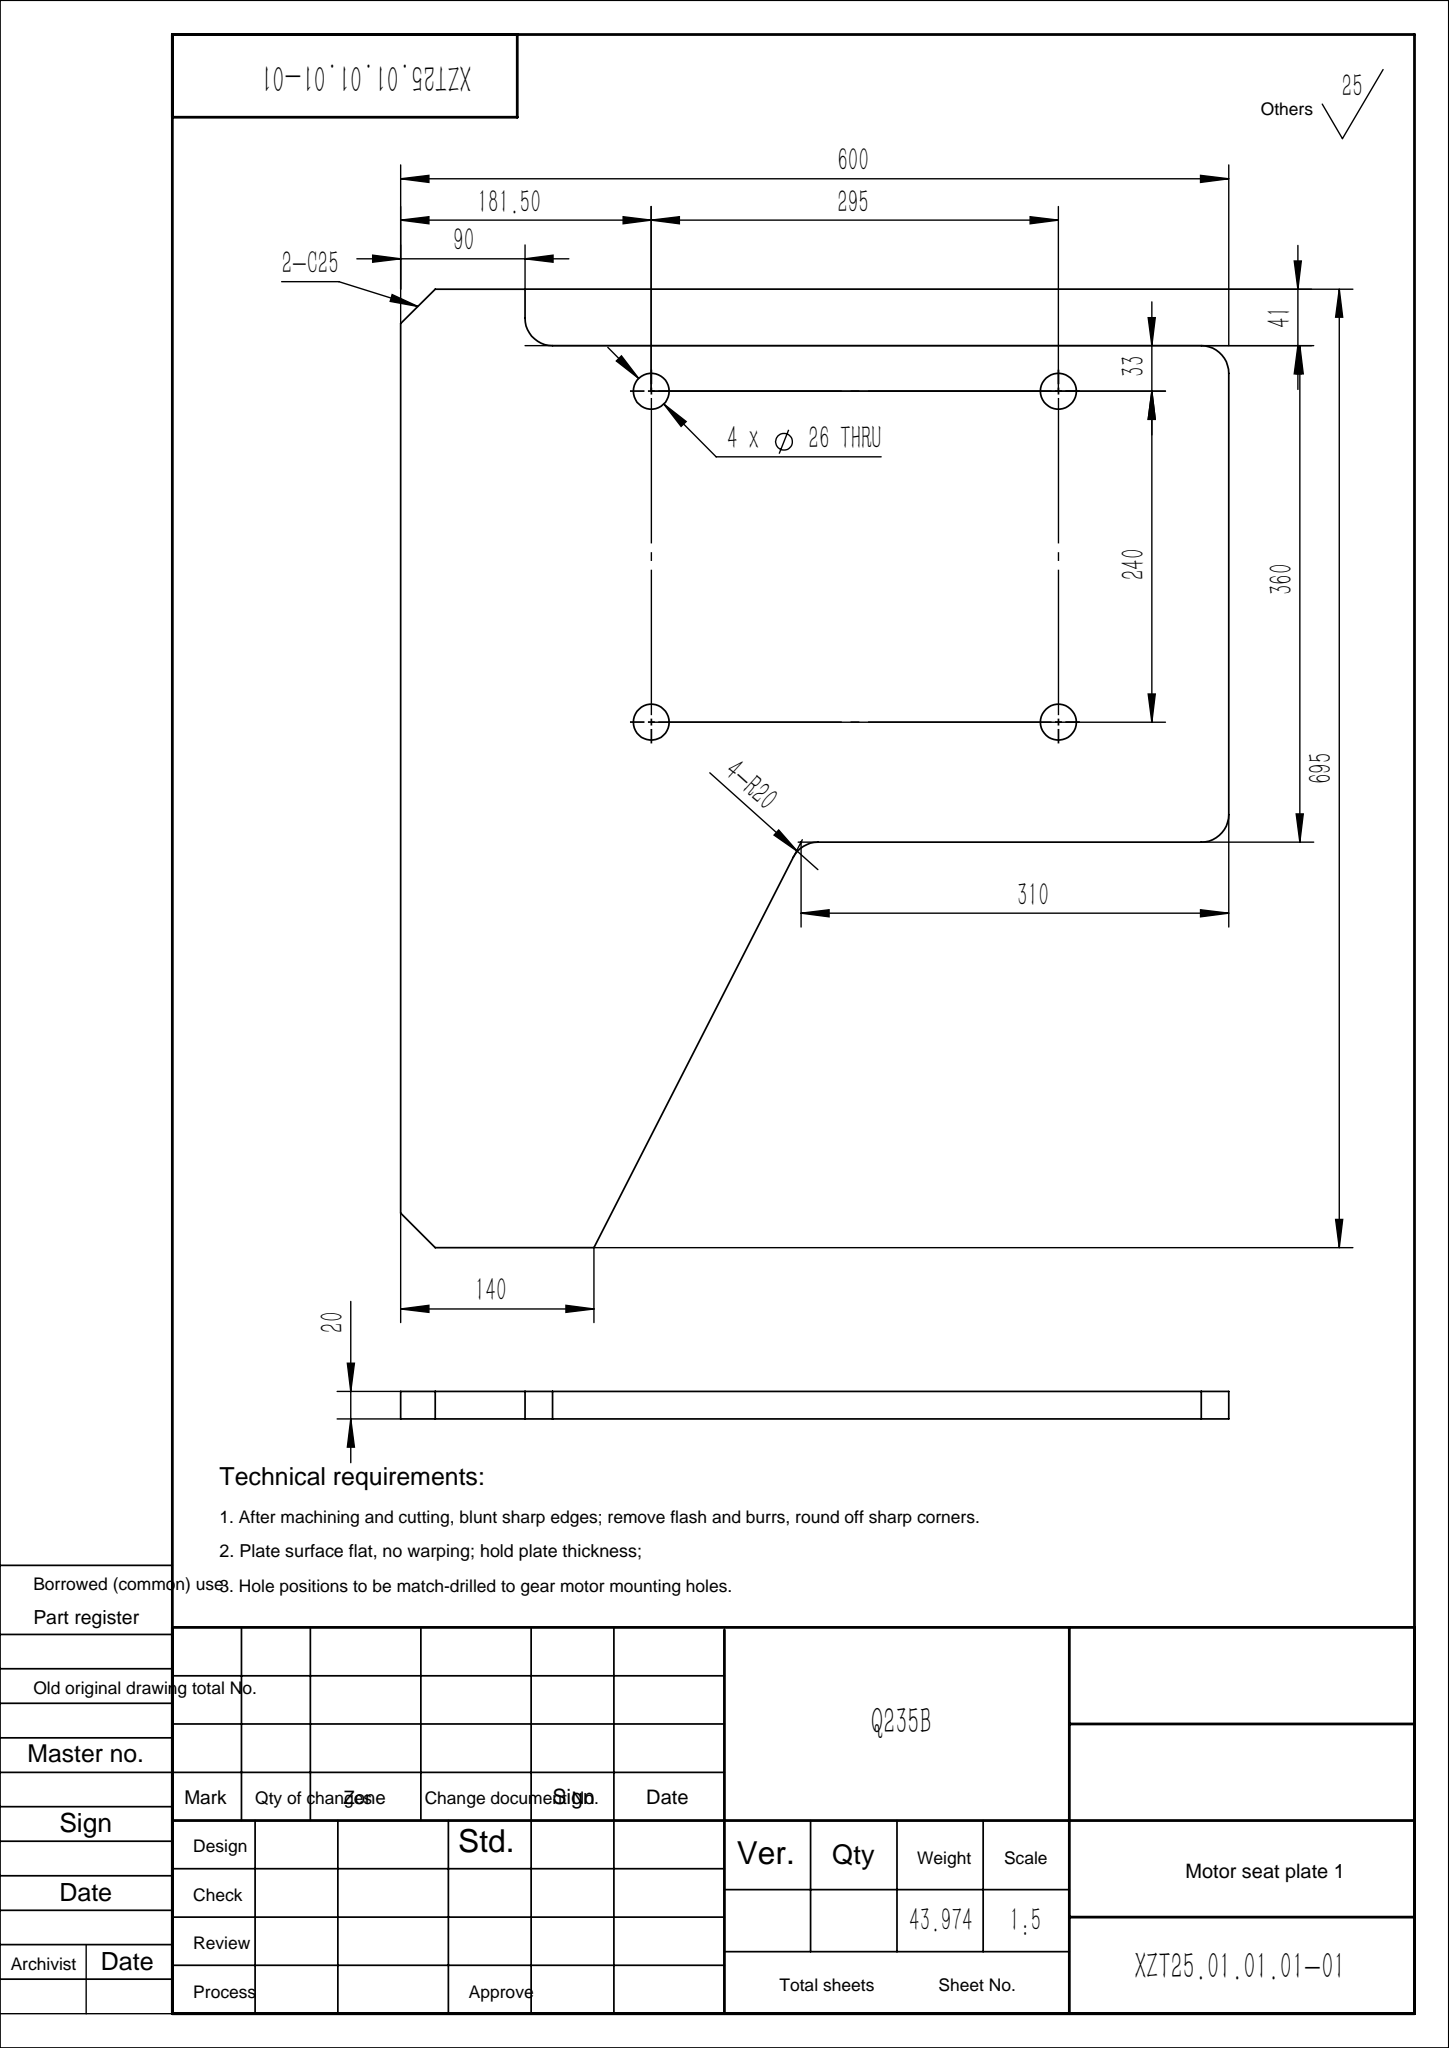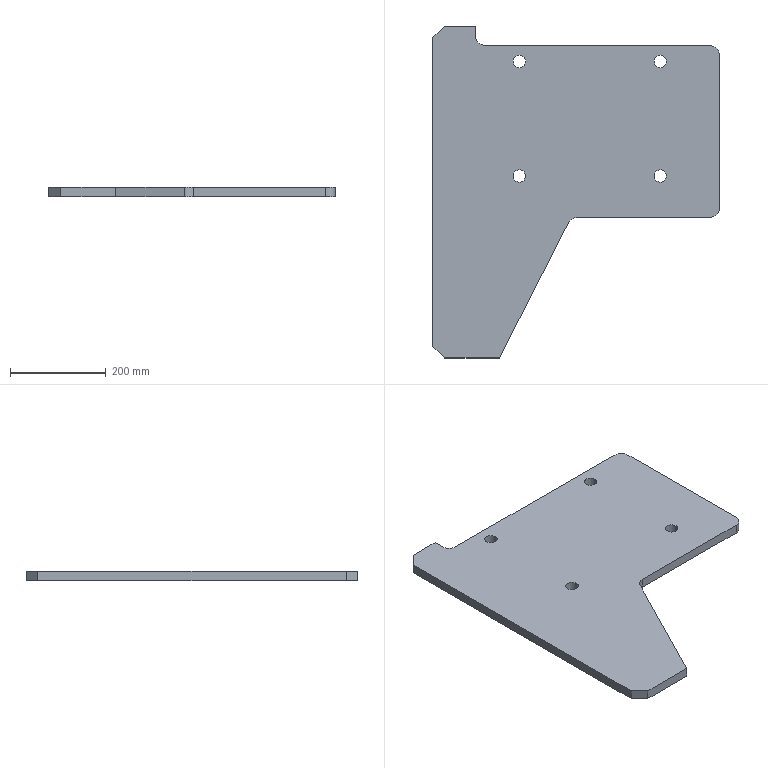Part | SolidWorks | features Chamfer 1, Extrusion 1, Fillet 1, HoleWzd 1 | 1 solid | 24 faces | box 600 x 695 x 20 mm | volume 5601812 mm3 | cylinder 12 | plane 12 | commonest cylinder face diameters 26 x8 40 x4
STEP:
#1=CARTESIAN_POINT('',(194.5,621.,-10.));
#2=VERTEX_POINT('',#1);
#3=CARTESIAN_POINT('',(168.5,621.,-10.));
#4=VERTEX_POINT('',#3);
#5=CARTESIAN_POINT('',(181.5,621.,-10.));
#6=DIRECTION('',(0.,0.,-1.));
#7=DIRECTION('',(-1.,0.,0.));
#8=AXIS2_PLACEMENT_3D('',#5,#6,#7);
#9=CIRCLE('',#8,13.);
#10=EDGE_CURVE('',#2,#4,#9,.T.);
#11=ORIENTED_EDGE('',*,*,#10,.T.);
#12=CARTESIAN_POINT('',(168.5,621.,10.));
#13=VERTEX_POINT('',#12);
#14=CARTESIAN_POINT('',(168.5,621.,10.));
#15=DIRECTION('',(0.,0.,1.));
#16=VECTOR('',#15,1000.);
#17=LINE('',#14,#16);
#18=EDGE_CURVE('',#4,#13,#17,.T.);
#19=ORIENTED_EDGE('',*,*,#18,.T.);
#20=CARTESIAN_POINT('',(194.5,621.,10.));
#21=VERTEX_POINT('',#20);
#22=CARTESIAN_POINT('',(181.5,621.,10.));
#23=DIRECTION('',(0.,0.,1.));
#24=DIRECTION('',(1.,0.,0.));
#25=AXIS2_PLACEMENT_3D('',#22,#23,#24);
#26=CIRCLE('',#25,13.);
#27=EDGE_CURVE('',#13,#21,#26,.T.);
#28=ORIENTED_EDGE('',*,*,#27,.T.);
#29=CARTESIAN_POINT('',(194.5,621.,10.));
#30=DIRECTION('',(0.,0.,1.));
#31=VECTOR('',#30,1000.);
#32=LINE('',#29,#31);
#33=EDGE_CURVE('',#2,#21,#32,.T.);
#34=ORIENTED_EDGE('',*,*,#33,.F.);
#35=EDGE_LOOP('',(#11,#19,#28,#34));
#36=FACE_OUTER_BOUND('',#35,.T.);
#37=CARTESIAN_POINT('',(181.5,621.,10.));
#38=DIRECTION('',(0.,0.,1.));
#39=DIRECTION('',(1.,0.,0.));
#40=AXIS2_PLACEMENT_3D('',#37,#38,#39);
#41=CYLINDRICAL_SURFACE('',#40,13.);
#42=ADVANCED_FACE('',(#36),#41,.F.);
#43=CARTESIAN_POINT('',(489.5,621.,-10.));
#44=VERTEX_POINT('',#43);
#45=CARTESIAN_POINT('',(463.5,621.,-10.));
#46=VERTEX_POINT('',#45);
#47=CARTESIAN_POINT('',(476.5,621.,-10.));
#48=DIRECTION('',(0.,0.,-1.));
#49=DIRECTION('',(-1.,0.,0.));
#50=AXIS2_PLACEMENT_3D('',#47,#48,#49);
#51=CIRCLE('',#50,13.);
#52=EDGE_CURVE('',#44,#46,#51,.T.);
#53=ORIENTED_EDGE('',*,*,#52,.T.);
#54=CARTESIAN_POINT('',(463.5,621.,10.));
#55=VERTEX_POINT('',#54);
#56=CARTESIAN_POINT('',(463.5,621.,10.));
#57=DIRECTION('',(0.,0.,1.));
#58=VECTOR('',#57,1000.);
#59=LINE('',#56,#58);
#60=EDGE_CURVE('',#46,#55,#59,.T.);
#61=ORIENTED_EDGE('',*,*,#60,.T.);
#62=CARTESIAN_POINT('',(489.5,621.,10.));
#63=VERTEX_POINT('',#62);
#64=CARTESIAN_POINT('',(476.5,621.,10.));
#65=DIRECTION('',(0.,0.,1.));
#66=DIRECTION('',(1.,0.,0.));
#67=AXIS2_PLACEMENT_3D('',#64,#65,#66);
#68=CIRCLE('',#67,13.);
#69=EDGE_CURVE('',#55,#63,#68,.T.);
#70=ORIENTED_EDGE('',*,*,#69,.T.);
#71=CARTESIAN_POINT('',(489.5,621.,10.));
#72=DIRECTION('',(0.,0.,1.));
#73=VECTOR('',#72,1000.);
#74=LINE('',#71,#73);
#75=EDGE_CURVE('',#44,#63,#74,.T.);
#76=ORIENTED_EDGE('',*,*,#75,.F.);
#77=EDGE_LOOP('',(#53,#61,#70,#76));
#78=FACE_OUTER_BOUND('',#77,.T.);
#79=CARTESIAN_POINT('',(476.5,621.,10.));
#80=DIRECTION('',(0.,0.,1.));
#81=DIRECTION('',(1.,0.,0.));
#82=AXIS2_PLACEMENT_3D('',#79,#80,#81);
#83=CYLINDRICAL_SURFACE('',#82,13.);
#84=ADVANCED_FACE('',(#78),#83,.F.);
#85=CARTESIAN_POINT('',(489.5,381.,-10.));
#86=VERTEX_POINT('',#85);
#87=CARTESIAN_POINT('',(463.5,381.,-10.));
#88=VERTEX_POINT('',#87);
#89=CARTESIAN_POINT('',(476.5,381.,-10.));
#90=DIRECTION('',(0.,0.,-1.));
#91=DIRECTION('',(-1.,0.,0.));
#92=AXIS2_PLACEMENT_3D('',#89,#90,#91);
#93=CIRCLE('',#92,13.);
#94=EDGE_CURVE('',#86,#88,#93,.T.);
#95=ORIENTED_EDGE('',*,*,#94,.T.);
#96=CARTESIAN_POINT('',(463.5,381.,10.));
#97=VERTEX_POINT('',#96);
#98=CARTESIAN_POINT('',(463.5,381.,10.));
#99=DIRECTION('',(0.,0.,1.));
#100=VECTOR('',#99,1000.);
#101=LINE('',#98,#100);
#102=EDGE_CURVE('',#88,#97,#101,.T.);
#103=ORIENTED_EDGE('',*,*,#102,.T.);
#104=CARTESIAN_POINT('',(489.5,381.,10.));
#105=VERTEX_POINT('',#104);
#106=CARTESIAN_POINT('',(476.5,381.,10.));
#107=DIRECTION('',(0.,0.,1.));
#108=DIRECTION('',(1.,0.,0.));
#109=AXIS2_PLACEMENT_3D('',#106,#107,#108);
#110=CIRCLE('',#109,13.);
#111=EDGE_CURVE('',#97,#105,#110,.T.);
#112=ORIENTED_EDGE('',*,*,#111,.T.);
#113=CARTESIAN_POINT('',(489.5,381.,10.));
#114=DIRECTION('',(0.,0.,1.));
#115=VECTOR('',#114,1000.);
#116=LINE('',#113,#115);
#117=EDGE_CURVE('',#86,#105,#116,.T.);
#118=ORIENTED_EDGE('',*,*,#117,.F.);
#119=EDGE_LOOP('',(#95,#103,#112,#118));
#120=FACE_OUTER_BOUND('',#119,.T.);
#121=CARTESIAN_POINT('',(476.5,381.,10.));
#122=DIRECTION('',(0.,0.,1.));
#123=DIRECTION('',(1.,0.,0.));
#124=AXIS2_PLACEMENT_3D('',#121,#122,#123);
#125=CYLINDRICAL_SURFACE('',#124,13.);
#126=ADVANCED_FACE('',(#120),#125,.F.);
#127=CARTESIAN_POINT('',(194.5,381.,-10.));
#128=VERTEX_POINT('',#127);
#129=CARTESIAN_POINT('',(168.5,381.,-10.));
#130=VERTEX_POINT('',#129);
#131=CARTESIAN_POINT('',(181.5,381.,-10.));
#132=DIRECTION('',(0.,0.,-1.));
#133=DIRECTION('',(-1.,0.,0.));
#134=AXIS2_PLACEMENT_3D('',#131,#132,#133);
#135=CIRCLE('',#134,13.);
#136=EDGE_CURVE('',#128,#130,#135,.T.);
#137=ORIENTED_EDGE('',*,*,#136,.T.);
#138=CARTESIAN_POINT('',(168.5,381.,10.));
#139=VERTEX_POINT('',#138);
#140=CARTESIAN_POINT('',(168.5,381.,10.));
#141=DIRECTION('',(0.,0.,1.));
#142=VECTOR('',#141,1000.);
#143=LINE('',#140,#142);
#144=EDGE_CURVE('',#130,#139,#143,.T.);
#145=ORIENTED_EDGE('',*,*,#144,.T.);
#146=CARTESIAN_POINT('',(194.5,381.,10.));
#147=VERTEX_POINT('',#146);
#148=CARTESIAN_POINT('',(181.5,381.,10.));
#149=DIRECTION('',(0.,0.,1.));
#150=DIRECTION('',(1.,0.,0.));
#151=AXIS2_PLACEMENT_3D('',#148,#149,#150);
#152=CIRCLE('',#151,13.);
#153=EDGE_CURVE('',#139,#147,#152,.T.);
#154=ORIENTED_EDGE('',*,*,#153,.T.);
#155=CARTESIAN_POINT('',(194.5,381.,10.));
#156=DIRECTION('',(0.,0.,1.));
#157=VECTOR('',#156,1000.);
#158=LINE('',#155,#157);
#159=EDGE_CURVE('',#128,#147,#158,.T.);
#160=ORIENTED_EDGE('',*,*,#159,.F.);
#161=EDGE_LOOP('',(#137,#145,#154,#160));
#162=FACE_OUTER_BOUND('',#161,.T.);
#163=CARTESIAN_POINT('',(181.5,381.,10.));
#164=DIRECTION('',(0.,0.,1.));
#165=DIRECTION('',(1.,0.,0.));
#166=AXIS2_PLACEMENT_3D('',#163,#164,#165);
#167=CYLINDRICAL_SURFACE('',#166,13.);
#168=ADVANCED_FACE('',(#162),#167,.F.);
#169=CARTESIAN_POINT('',(476.5,381.,10.));
#170=DIRECTION('',(0.,0.,1.));
#171=DIRECTION('',(1.,0.,0.));
#172=AXIS2_PLACEMENT_3D('',#169,#170,#171);
#173=CIRCLE('',#172,13.);
#174=EDGE_CURVE('',#105,#97,#173,.T.);
#175=ORIENTED_EDGE('',*,*,#174,.F.);
#176=ORIENTED_EDGE('',*,*,#111,.F.);
#177=EDGE_LOOP('',(#175,#176));
#178=FACE_BOUND('',#177,.T.);
#179=CARTESIAN_POINT('',(181.5,381.,10.));
#180=DIRECTION('',(0.,0.,1.));
#181=DIRECTION('',(1.,0.,0.));
#182=AXIS2_PLACEMENT_3D('',#179,#180,#181);
#183=CIRCLE('',#182,13.);
#184=EDGE_CURVE('',#147,#139,#183,.T.);
#185=ORIENTED_EDGE('',*,*,#184,.F.);
#186=ORIENTED_EDGE('',*,*,#153,.F.);
#187=EDGE_LOOP('',(#185,#186));
#188=FACE_BOUND('',#187,.T.);
#189=CARTESIAN_POINT('',(302.249,294.,10.));
#190=VERTEX_POINT('',#189);
#191=CARTESIAN_POINT('',(580.,294.,10.));
#192=VERTEX_POINT('',#191);
#193=CARTESIAN_POINT('',(600.,294.,10.));
#194=DIRECTION('',(1.,0.,0.));
#195=VECTOR('',#194,1000.);
#196=LINE('',#193,#195);
#197=EDGE_CURVE('',#190,#192,#196,.T.);
#198=ORIENTED_EDGE('',*,*,#197,.T.);
#199=CARTESIAN_POINT('',(600.,314.,10.));
#200=VERTEX_POINT('',#199);
#201=CARTESIAN_POINT('',(580.,314.,10.));
#202=DIRECTION('',(0.,0.,1.));
#203=DIRECTION('',(-1.,0.,0.));
#204=AXIS2_PLACEMENT_3D('',#201,#202,#203);
#205=CIRCLE('',#204,20.);
#206=EDGE_CURVE('',#192,#200,#205,.T.);
#207=ORIENTED_EDGE('',*,*,#206,.T.);
#208=CARTESIAN_POINT('',(600.,634.,10.));
#209=VERTEX_POINT('',#208);
#210=CARTESIAN_POINT('',(600.,654.,10.));
#211=DIRECTION('',(0.,1.,0.));
#212=VECTOR('',#211,1000.);
#213=LINE('',#210,#212);
#214=EDGE_CURVE('',#200,#209,#213,.T.);
#215=ORIENTED_EDGE('',*,*,#214,.T.);
#216=CARTESIAN_POINT('',(580.,654.,10.));
#217=VERTEX_POINT('',#216);
#218=CARTESIAN_POINT('',(580.,634.,10.));
#219=DIRECTION('',(0.,0.,1.));
#220=DIRECTION('',(-1.,0.,0.));
#221=AXIS2_PLACEMENT_3D('',#218,#219,#220);
#222=CIRCLE('',#221,20.);
#223=EDGE_CURVE('',#209,#217,#222,.T.);
#224=ORIENTED_EDGE('',*,*,#223,.T.);
#225=CARTESIAN_POINT('',(110.,654.,10.));
#226=VERTEX_POINT('',#225);
#227=CARTESIAN_POINT('',(90.,654.,10.));
#228=DIRECTION('',(-1.,0.,0.));
#229=VECTOR('',#228,1000.);
#230=LINE('',#227,#229);
#231=EDGE_CURVE('',#217,#226,#230,.T.);
#232=ORIENTED_EDGE('',*,*,#231,.T.);
#233=CARTESIAN_POINT('',(90.,674.,10.));
#234=VERTEX_POINT('',#233);
#235=CARTESIAN_POINT('',(110.,674.,10.));
#236=DIRECTION('',(0.,0.,-1.));
#237=DIRECTION('',(-1.,0.,0.));
#238=AXIS2_PLACEMENT_3D('',#235,#236,#237);
#239=CIRCLE('',#238,20.);
#240=EDGE_CURVE('',#226,#234,#239,.T.);
#241=ORIENTED_EDGE('',*,*,#240,.T.);
#242=CARTESIAN_POINT('',(90.,695.,10.));
#243=VERTEX_POINT('',#242);
#244=CARTESIAN_POINT('',(90.,695.,10.));
#245=DIRECTION('',(0.,1.,0.));
#246=VECTOR('',#245,1000.);
#247=LINE('',#244,#246);
#248=EDGE_CURVE('',#234,#243,#247,.T.);
#249=ORIENTED_EDGE('',*,*,#248,.T.);
#250=CARTESIAN_POINT('',(25.,695.,10.));
#251=VERTEX_POINT('',#250);
#252=CARTESIAN_POINT('',(0.,695.,10.));
#253=DIRECTION('',(-1.,0.,0.));
#254=VECTOR('',#253,1000.);
#255=LINE('',#252,#254);
#256=EDGE_CURVE('',#243,#251,#255,.T.);
#257=ORIENTED_EDGE('',*,*,#256,.T.);
#258=CARTESIAN_POINT('',(0.,670.,10.));
#259=VERTEX_POINT('',#258);
#260=CARTESIAN_POINT('',(0.,670.,10.));
#261=DIRECTION('',(-0.7071,-0.7071,0.));
#262=VECTOR('',#261,1000.);
#263=LINE('',#260,#262);
#264=EDGE_CURVE('',#251,#259,#263,.T.);
#265=ORIENTED_EDGE('',*,*,#264,.T.);
#266=CARTESIAN_POINT('',(0.,25.,10.));
#267=VERTEX_POINT('',#266);
#268=CARTESIAN_POINT('',(0.,0.,10.));
#269=DIRECTION('',(0.,-1.,0.));
#270=VECTOR('',#269,1000.);
#271=LINE('',#268,#270);
#272=EDGE_CURVE('',#259,#267,#271,.T.);
#273=ORIENTED_EDGE('',*,*,#272,.T.);
#274=CARTESIAN_POINT('',(25.,0.,10.));
#275=VERTEX_POINT('',#274);
#276=CARTESIAN_POINT('',(25.,0.,10.));
#277=DIRECTION('',(0.7071,-0.7071,0.));
#278=VECTOR('',#277,1000.);
#279=LINE('',#276,#278);
#280=EDGE_CURVE('',#267,#275,#279,.T.);
#281=ORIENTED_EDGE('',*,*,#280,.T.);
#282=CARTESIAN_POINT('',(140.,0.,10.));
#283=VERTEX_POINT('',#282);
#284=CARTESIAN_POINT('',(140.,0.,10.));
#285=DIRECTION('',(1.,0.,0.));
#286=VECTOR('',#285,1000.);
#287=LINE('',#284,#286);
#288=EDGE_CURVE('',#275,#283,#287,.T.);
#289=ORIENTED_EDGE('',*,*,#288,.T.);
#290=CARTESIAN_POINT('',(284.433,283.089,10.));
#291=VERTEX_POINT('',#290);
#292=CARTESIAN_POINT('',(290.,294.,10.));
#293=DIRECTION('',(0.4545,0.8908,0.));
#294=VECTOR('',#293,1000.);
#295=LINE('',#292,#294);
#296=EDGE_CURVE('',#283,#291,#295,.T.);
#297=ORIENTED_EDGE('',*,*,#296,.T.);
#298=CARTESIAN_POINT('',(302.249,274.,10.));
#299=DIRECTION('',(0.,0.,-1.));
#300=DIRECTION('',(-1.,0.,0.));
#301=AXIS2_PLACEMENT_3D('',#298,#299,#300);
#302=CIRCLE('',#301,20.);
#303=EDGE_CURVE('',#291,#190,#302,.T.);
#304=ORIENTED_EDGE('',*,*,#303,.T.);
#305=EDGE_LOOP('',(#198,#207,#215,#224,#232,#241,#249,#257,#265,#273,#281,#289,#297,#304));
#306=FACE_OUTER_BOUND('',#305,.T.);
#307=CARTESIAN_POINT('',(476.5,621.,10.));
#308=DIRECTION('',(0.,0.,1.));
#309=DIRECTION('',(1.,0.,0.));
#310=AXIS2_PLACEMENT_3D('',#307,#308,#309);
#311=CIRCLE('',#310,13.);
#312=EDGE_CURVE('',#63,#55,#311,.T.);
#313=ORIENTED_EDGE('',*,*,#312,.F.);
#314=ORIENTED_EDGE('',*,*,#69,.F.);
#315=EDGE_LOOP('',(#313,#314));
#316=FACE_BOUND('',#315,.T.);
#317=CARTESIAN_POINT('',(181.5,621.,10.));
#318=DIRECTION('',(0.,0.,1.));
#319=DIRECTION('',(1.,0.,0.));
#320=AXIS2_PLACEMENT_3D('',#317,#318,#319);
#321=CIRCLE('',#320,13.);
#322=EDGE_CURVE('',#21,#13,#321,.T.);
#323=ORIENTED_EDGE('',*,*,#322,.F.);
#324=ORIENTED_EDGE('',*,*,#27,.F.);
#325=EDGE_LOOP('',(#323,#324));
#326=FACE_BOUND('',#325,.T.);
#327=CARTESIAN_POINT('',(0.,0.,10.));
#328=DIRECTION('',(0.,0.,-1.));
#329=DIRECTION('',(-1.,0.,0.));
#330=AXIS2_PLACEMENT_3D('',#327,#328,#329);
#331=PLANE('',#330);
#332=ADVANCED_FACE('',(#178,#188,#306,#316,#326),#331,.F.);
#333=ORIENTED_EDGE('',*,*,#288,.F.);
#334=CARTESIAN_POINT('',(25.,0.,-10.));
#335=VERTEX_POINT('',#334);
#336=CARTESIAN_POINT('',(25.,0.,10.));
#337=DIRECTION('',(0.,0.,-1.));
#338=VECTOR('',#337,1000.);
#339=LINE('',#336,#338);
#340=EDGE_CURVE('',#275,#335,#339,.T.);
#341=ORIENTED_EDGE('',*,*,#340,.T.);
#342=CARTESIAN_POINT('',(140.,0.,-10.));
#343=VERTEX_POINT('',#342);
#344=CARTESIAN_POINT('',(140.,0.,-10.));
#345=DIRECTION('',(1.,0.,0.));
#346=VECTOR('',#345,1000.);
#347=LINE('',#344,#346);
#348=EDGE_CURVE('',#335,#343,#347,.T.);
#349=ORIENTED_EDGE('',*,*,#348,.T.);
#350=CARTESIAN_POINT('',(140.,0.,10.));
#351=DIRECTION('',(0.,0.,-1.));
#352=VECTOR('',#351,1000.);
#353=LINE('',#350,#352);
#354=EDGE_CURVE('',#283,#343,#353,.T.);
#355=ORIENTED_EDGE('',*,*,#354,.F.);
#356=EDGE_LOOP('',(#333,#341,#349,#355));
#357=FACE_OUTER_BOUND('',#356,.T.);
#358=CARTESIAN_POINT('',(140.,0.,10.));
#359=DIRECTION('',(0.,1.,0.));
#360=DIRECTION('',(0.,0.,1.));
#361=AXIS2_PLACEMENT_3D('',#358,#359,#360);
#362=PLANE('',#361);
#363=ADVANCED_FACE('',(#357),#362,.F.);
#364=CARTESIAN_POINT('',(284.433,283.089,-10.));
#365=VERTEX_POINT('',#364);
#366=CARTESIAN_POINT('',(290.,294.,-10.));
#367=DIRECTION('',(0.4545,0.8908,0.));
#368=VECTOR('',#367,1000.);
#369=LINE('',#366,#368);
#370=EDGE_CURVE('',#343,#365,#369,.T.);
#371=ORIENTED_EDGE('',*,*,#370,.T.);
#372=CARTESIAN_POINT('',(284.433,283.089,10.));
#373=DIRECTION('',(0.,0.,1.));
#374=VECTOR('',#373,1000.);
#375=LINE('',#372,#374);
#376=EDGE_CURVE('',#365,#291,#375,.T.);
#377=ORIENTED_EDGE('',*,*,#376,.T.);
#378=ORIENTED_EDGE('',*,*,#296,.F.);
#379=ORIENTED_EDGE('',*,*,#354,.T.);
#380=EDGE_LOOP('',(#371,#377,#378,#379));
#381=FACE_OUTER_BOUND('',#380,.T.);
#382=CARTESIAN_POINT('',(290.,294.,10.));
#383=DIRECTION('',(-0.8908,0.4545,0.));
#384=DIRECTION('',(-0.4545,-0.8908,0.));
#385=AXIS2_PLACEMENT_3D('',#382,#383,#384);
#386=PLANE('',#385);
#387=ADVANCED_FACE('',(#381),#386,.F.);
#388=CARTESIAN_POINT('',(302.249,294.,-10.));
#389=VERTEX_POINT('',#388);
#390=CARTESIAN_POINT('',(580.,294.,-10.));
#391=VERTEX_POINT('',#390);
#392=CARTESIAN_POINT('',(600.,294.,-10.));
#393=DIRECTION('',(1.,0.,0.));
#394=VECTOR('',#393,1000.);
#395=LINE('',#392,#394);
#396=EDGE_CURVE('',#389,#391,#395,.T.);
#397=ORIENTED_EDGE('',*,*,#396,.T.);
#398=CARTESIAN_POINT('',(580.,294.,10.));
#399=DIRECTION('',(0.,0.,1.));
#400=VECTOR('',#399,1000.);
#401=LINE('',#398,#400);
#402=EDGE_CURVE('',#391,#192,#401,.T.);
#403=ORIENTED_EDGE('',*,*,#402,.T.);
#404=ORIENTED_EDGE('',*,*,#197,.F.);
#405=CARTESIAN_POINT('',(302.249,294.,-10.));
#406=DIRECTION('',(0.,0.,-1.));
#407=VECTOR('',#406,1000.);
#408=LINE('',#405,#407);
#409=EDGE_CURVE('',#190,#389,#408,.T.);
#410=ORIENTED_EDGE('',*,*,#409,.T.);
#411=EDGE_LOOP('',(#397,#403,#404,#410));
#412=FACE_OUTER_BOUND('',#411,.T.);
#413=CARTESIAN_POINT('',(600.,294.,10.));
#414=DIRECTION('',(0.,1.,0.));
#415=DIRECTION('',(-1.,0.,0.));
#416=AXIS2_PLACEMENT_3D('',#413,#414,#415);
#417=PLANE('',#416);
#418=ADVANCED_FACE('',(#412),#417,.F.);
#419=ORIENTED_EDGE('',*,*,#214,.F.);
#420=CARTESIAN_POINT('',(600.,314.,-10.));
#421=VERTEX_POINT('',#420);
#422=CARTESIAN_POINT('',(600.,314.,10.));
#423=DIRECTION('',(0.,0.,-1.));
#424=VECTOR('',#423,1000.);
#425=LINE('',#422,#424);
#426=EDGE_CURVE('',#200,#421,#425,.T.);
#427=ORIENTED_EDGE('',*,*,#426,.T.);
#428=CARTESIAN_POINT('',(600.,634.,-10.));
#429=VERTEX_POINT('',#428);
#430=CARTESIAN_POINT('',(600.,654.,-10.));
#431=DIRECTION('',(0.,1.,0.));
#432=VECTOR('',#431,1000.);
#433=LINE('',#430,#432);
#434=EDGE_CURVE('',#421,#429,#433,.T.);
#435=ORIENTED_EDGE('',*,*,#434,.T.);
#436=CARTESIAN_POINT('',(600.,634.,10.));
#437=DIRECTION('',(0.,0.,1.));
#438=VECTOR('',#437,1000.);
#439=LINE('',#436,#438);
#440=EDGE_CURVE('',#429,#209,#439,.T.);
#441=ORIENTED_EDGE('',*,*,#440,.T.);
#442=EDGE_LOOP('',(#419,#427,#435,#441));
#443=FACE_OUTER_BOUND('',#442,.T.);
#444=CARTESIAN_POINT('',(600.,654.,10.));
#445=DIRECTION('',(-1.,0.,0.));
#446=DIRECTION('',(0.,0.,1.));
#447=AXIS2_PLACEMENT_3D('',#444,#445,#446);
#448=PLANE('',#447);
#449=ADVANCED_FACE('',(#443),#448,.F.);
#450=ORIENTED_EDGE('',*,*,#231,.F.);
#451=CARTESIAN_POINT('',(580.,654.,-10.));
#452=VERTEX_POINT('',#451);
#453=CARTESIAN_POINT('',(580.,654.,10.));
#454=DIRECTION('',(0.,0.,-1.));
#455=VECTOR('',#454,1000.);
#456=LINE('',#453,#455);
#457=EDGE_CURVE('',#217,#452,#456,.T.);
#458=ORIENTED_EDGE('',*,*,#457,.T.);
#459=CARTESIAN_POINT('',(110.,654.,-10.));
#460=VERTEX_POINT('',#459);
#461=CARTESIAN_POINT('',(90.,654.,-10.));
#462=DIRECTION('',(-1.,0.,0.));
#463=VECTOR('',#462,1000.);
#464=LINE('',#461,#463);
#465=EDGE_CURVE('',#452,#460,#464,.T.);
#466=ORIENTED_EDGE('',*,*,#465,.T.);
#467=CARTESIAN_POINT('',(110.,654.,10.));
#468=DIRECTION('',(0.,0.,1.));
#469=VECTOR('',#468,1000.);
#470=LINE('',#467,#469);
#471=EDGE_CURVE('',#460,#226,#470,.T.);
#472=ORIENTED_EDGE('',*,*,#471,.T.);
#473=EDGE_LOOP('',(#450,#458,#466,#472));
#474=FACE_OUTER_BOUND('',#473,.T.);
#475=CARTESIAN_POINT('',(90.,654.,10.));
#476=DIRECTION('',(0.,-1.,0.));
#477=DIRECTION('',(0.,0.,-1.));
#478=AXIS2_PLACEMENT_3D('',#475,#476,#477);
#479=PLANE('',#478);
#480=ADVANCED_FACE('',(#474),#479,.F.);
#481=ORIENTED_EDGE('',*,*,#248,.F.);
#482=CARTESIAN_POINT('',(90.,674.,-10.));
#483=VERTEX_POINT('',#482);
#484=CARTESIAN_POINT('',(90.,674.,-10.));
#485=DIRECTION('',(0.,0.,-1.));
#486=VECTOR('',#485,1000.);
#487=LINE('',#484,#486);
#488=EDGE_CURVE('',#234,#483,#487,.T.);
#489=ORIENTED_EDGE('',*,*,#488,.T.);
#490=CARTESIAN_POINT('',(90.,695.,-10.));
#491=VERTEX_POINT('',#490);
#492=CARTESIAN_POINT('',(90.,695.,-10.));
#493=DIRECTION('',(0.,1.,0.));
#494=VECTOR('',#493,1000.);
#495=LINE('',#492,#494);
#496=EDGE_CURVE('',#483,#491,#495,.T.);
#497=ORIENTED_EDGE('',*,*,#496,.T.);
#498=CARTESIAN_POINT('',(90.,695.,10.));
#499=DIRECTION('',(0.,0.,-1.));
#500=VECTOR('',#499,1000.);
#501=LINE('',#498,#500);
#502=EDGE_CURVE('',#243,#491,#501,.T.);
#503=ORIENTED_EDGE('',*,*,#502,.F.);
#504=EDGE_LOOP('',(#481,#489,#497,#503));
#505=FACE_OUTER_BOUND('',#504,.T.);
#506=CARTESIAN_POINT('',(90.,695.,10.));
#507=DIRECTION('',(-1.,0.,0.));
#508=DIRECTION('',(0.,-1.,0.));
#509=AXIS2_PLACEMENT_3D('',#506,#507,#508);
#510=PLANE('',#509);
#511=ADVANCED_FACE('',(#505),#510,.F.);
#512=CARTESIAN_POINT('',(25.,695.,-10.));
#513=VERTEX_POINT('',#512);
#514=CARTESIAN_POINT('',(0.,695.,-10.));
#515=DIRECTION('',(-1.,0.,0.));
#516=VECTOR('',#515,1000.);
#517=LINE('',#514,#516);
#518=EDGE_CURVE('',#491,#513,#517,.T.);
#519=ORIENTED_EDGE('',*,*,#518,.T.);
#520=CARTESIAN_POINT('',(25.,695.,10.));
#521=DIRECTION('',(0.,0.,1.));
#522=VECTOR('',#521,1000.);
#523=LINE('',#520,#522);
#524=EDGE_CURVE('',#513,#251,#523,.T.);
#525=ORIENTED_EDGE('',*,*,#524,.T.);
#526=ORIENTED_EDGE('',*,*,#256,.F.);
#527=ORIENTED_EDGE('',*,*,#502,.T.);
#528=EDGE_LOOP('',(#519,#525,#526,#527));
#529=FACE_OUTER_BOUND('',#528,.T.);
#530=CARTESIAN_POINT('',(0.,695.,10.));
#531=DIRECTION('',(0.,-1.,0.));
#532=DIRECTION('',(0.,0.,-1.));
#533=AXIS2_PLACEMENT_3D('',#530,#531,#532);
#534=PLANE('',#533);
#535=ADVANCED_FACE('',(#529),#534,.F.);
#536=CARTESIAN_POINT('',(0.,670.,-10.));
#537=VERTEX_POINT('',#536);
#538=CARTESIAN_POINT('',(0.,25.,-10.));
#539=VERTEX_POINT('',#538);
#540=CARTESIAN_POINT('',(0.,0.,-10.));
#541=DIRECTION('',(0.,-1.,0.));
#542=VECTOR('',#541,1000.);
#543=LINE('',#540,#542);
#544=EDGE_CURVE('',#537,#539,#543,.T.);
#545=ORIENTED_EDGE('',*,*,#544,.T.);
#546=CARTESIAN_POINT('',(0.,25.,10.));
#547=DIRECTION('',(0.,0.,1.));
#548=VECTOR('',#547,1000.);
#549=LINE('',#546,#548);
#550=EDGE_CURVE('',#539,#267,#549,.T.);
#551=ORIENTED_EDGE('',*,*,#550,.T.);
#552=ORIENTED_EDGE('',*,*,#272,.F.);
#553=CARTESIAN_POINT('',(0.,670.,10.));
#554=DIRECTION('',(0.,0.,-1.));
#555=VECTOR('',#554,1000.);
#556=LINE('',#553,#555);
#557=EDGE_CURVE('',#259,#537,#556,.T.);
#558=ORIENTED_EDGE('',*,*,#557,.T.);
#559=EDGE_LOOP('',(#545,#551,#552,#558));
#560=FACE_OUTER_BOUND('',#559,.T.);
#561=CARTESIAN_POINT('',(0.,0.,10.));
#562=DIRECTION('',(1.,0.,0.));
#563=DIRECTION('',(0.,0.,-1.));
#564=AXIS2_PLACEMENT_3D('',#561,#562,#563);
#565=PLANE('',#564);
#566=ADVANCED_FACE('',(#560),#565,.F.);
#567=ORIENTED_EDGE('',*,*,#10,.F.);
#568=CARTESIAN_POINT('',(181.5,621.,-10.));
#569=DIRECTION('',(0.,0.,-1.));
#570=DIRECTION('',(-1.,0.,0.));
#571=AXIS2_PLACEMENT_3D('',#568,#569,#570);
#572=CIRCLE('',#571,13.);
#573=EDGE_CURVE('',#4,#2,#572,.T.);
#574=ORIENTED_EDGE('',*,*,#573,.F.);
#575=EDGE_LOOP('',(#567,#574));
#576=FACE_BOUND('',#575,.T.);
#577=ORIENTED_EDGE('',*,*,#52,.F.);
#578=CARTESIAN_POINT('',(476.5,621.,-10.));
#579=DIRECTION('',(0.,0.,-1.));
#580=DIRECTION('',(-1.,0.,0.));
#581=AXIS2_PLACEMENT_3D('',#578,#579,#580);
#582=CIRCLE('',#581,13.);
#583=EDGE_CURVE('',#46,#44,#582,.T.);
#584=ORIENTED_EDGE('',*,*,#583,.F.);
#585=EDGE_LOOP('',(#577,#584));
#586=FACE_BOUND('',#585,.T.);
#587=ORIENTED_EDGE('',*,*,#94,.F.);
#588=CARTESIAN_POINT('',(476.5,381.,-10.));
#589=DIRECTION('',(0.,0.,-1.));
#590=DIRECTION('',(-1.,0.,0.));
#591=AXIS2_PLACEMENT_3D('',#588,#589,#590);
#592=CIRCLE('',#591,13.);
#593=EDGE_CURVE('',#88,#86,#592,.T.);
#594=ORIENTED_EDGE('',*,*,#593,.F.);
#595=EDGE_LOOP('',(#587,#594));
#596=FACE_BOUND('',#595,.T.);
#597=ORIENTED_EDGE('',*,*,#136,.F.);
#598=CARTESIAN_POINT('',(181.5,381.,-10.));
#599=DIRECTION('',(0.,0.,-1.));
#600=DIRECTION('',(-1.,0.,0.));
#601=AXIS2_PLACEMENT_3D('',#598,#599,#600);
#602=CIRCLE('',#601,13.);
#603=EDGE_CURVE('',#130,#128,#602,.T.);
#604=ORIENTED_EDGE('',*,*,#603,.F.);
#605=EDGE_LOOP('',(#597,#604));
#606=FACE_BOUND('',#605,.T.);
#607=ORIENTED_EDGE('',*,*,#434,.F.);
#608=CARTESIAN_POINT('',(580.,314.,-10.));
#609=DIRECTION('',(0.,0.,-1.));
#610=DIRECTION('',(-1.,0.,0.));
#611=AXIS2_PLACEMENT_3D('',#608,#609,#610);
#612=CIRCLE('',#611,20.);
#613=EDGE_CURVE('',#421,#391,#612,.T.);
#614=ORIENTED_EDGE('',*,*,#613,.T.);
#615=ORIENTED_EDGE('',*,*,#396,.F.);
#616=CARTESIAN_POINT('',(302.249,274.,-10.));
#617=DIRECTION('',(0.,0.,1.));
#618=DIRECTION('',(-1.,0.,0.));
#619=AXIS2_PLACEMENT_3D('',#616,#617,#618);
#620=CIRCLE('',#619,20.);
#621=EDGE_CURVE('',#389,#365,#620,.T.);
#622=ORIENTED_EDGE('',*,*,#621,.T.);
#623=ORIENTED_EDGE('',*,*,#370,.F.);
#624=ORIENTED_EDGE('',*,*,#348,.F.);
#625=CARTESIAN_POINT('',(12.5,12.5,-10.));
#626=DIRECTION('',(-0.7071,0.7071,0.));
#627=VECTOR('',#626,1000.);
#628=LINE('',#625,#627);
#629=EDGE_CURVE('',#335,#539,#628,.T.);
#630=ORIENTED_EDGE('',*,*,#629,.T.);
#631=ORIENTED_EDGE('',*,*,#544,.F.);
#632=CARTESIAN_POINT('',(-335.,335.,-10.));
#633=DIRECTION('',(0.7071,0.7071,0.));
#634=VECTOR('',#633,1000.);
#635=LINE('',#632,#634);
#636=EDGE_CURVE('',#537,#513,#635,.T.);
#637=ORIENTED_EDGE('',*,*,#636,.T.);
#638=ORIENTED_EDGE('',*,*,#518,.F.);
#639=ORIENTED_EDGE('',*,*,#496,.F.);
#640=CARTESIAN_POINT('',(110.,674.,-10.));
#641=DIRECTION('',(0.,0.,1.));
#642=DIRECTION('',(-1.,0.,0.));
#643=AXIS2_PLACEMENT_3D('',#640,#641,#642);
#644=CIRCLE('',#643,20.);
#645=EDGE_CURVE('',#483,#460,#644,.T.);
#646=ORIENTED_EDGE('',*,*,#645,.T.);
#647=ORIENTED_EDGE('',*,*,#465,.F.);
#648=CARTESIAN_POINT('',(580.,634.,-10.));
#649=DIRECTION('',(0.,0.,-1.));
#650=DIRECTION('',(-1.,0.,0.));
#651=AXIS2_PLACEMENT_3D('',#648,#649,#650);
#652=CIRCLE('',#651,20.);
#653=EDGE_CURVE('',#452,#429,#652,.T.);
#654=ORIENTED_EDGE('',*,*,#653,.T.);
#655=EDGE_LOOP('',(#607,#614,#615,#622,#623,#624,#630,#631,#637,#638,#639,#646,#647,#654));
#656=FACE_OUTER_BOUND('',#655,.T.);
#657=CARTESIAN_POINT('',(0.,0.,-10.));
#658=DIRECTION('',(0.,0.,-1.));
#659=DIRECTION('',(-1.,0.,0.));
#660=AXIS2_PLACEMENT_3D('',#657,#658,#659);
#661=PLANE('',#660);
#662=ADVANCED_FACE('',(#576,#586,#596,#606,#656),#661,.T.);
#663=ORIENTED_EDGE('',*,*,#280,.F.);
#664=ORIENTED_EDGE('',*,*,#550,.F.);
#665=ORIENTED_EDGE('',*,*,#629,.F.);
#666=ORIENTED_EDGE('',*,*,#340,.F.);
#667=EDGE_LOOP('',(#663,#664,#665,#666));
#668=FACE_OUTER_BOUND('',#667,.T.);
#669=CARTESIAN_POINT('',(25.,0.,10.));
#670=DIRECTION('',(0.7071,0.7071,0.));
#671=DIRECTION('',(0.,0.,-1.));
#672=AXIS2_PLACEMENT_3D('',#669,#670,#671);
#673=PLANE('',#672);
#674=ADVANCED_FACE('',(#668),#673,.F.);
#675=ORIENTED_EDGE('',*,*,#264,.F.);
#676=ORIENTED_EDGE('',*,*,#524,.F.);
#677=ORIENTED_EDGE('',*,*,#636,.F.);
#678=ORIENTED_EDGE('',*,*,#557,.F.);
#679=EDGE_LOOP('',(#675,#676,#677,#678));
#680=FACE_OUTER_BOUND('',#679,.T.);
#681=CARTESIAN_POINT('',(0.,670.,10.));
#682=DIRECTION('',(0.7071,-0.7071,0.));
#683=DIRECTION('',(0.,0.,-1.));
#684=AXIS2_PLACEMENT_3D('',#681,#682,#683);
#685=PLANE('',#684);
#686=ADVANCED_FACE('',(#680),#685,.F.);
#687=ORIENTED_EDGE('',*,*,#206,.F.);
#688=ORIENTED_EDGE('',*,*,#402,.F.);
#689=ORIENTED_EDGE('',*,*,#613,.F.);
#690=ORIENTED_EDGE('',*,*,#426,.F.);
#691=EDGE_LOOP('',(#687,#688,#689,#690));
#692=FACE_OUTER_BOUND('',#691,.T.);
#693=CARTESIAN_POINT('',(580.,314.,10.));
#694=DIRECTION('',(0.,0.,-1.));
#695=DIRECTION('',(-1.,0.,0.));
#696=AXIS2_PLACEMENT_3D('',#693,#694,#695);
#697=CYLINDRICAL_SURFACE('',#696,20.);
#698=ADVANCED_FACE('',(#692),#697,.T.);
#699=ORIENTED_EDGE('',*,*,#223,.F.);
#700=ORIENTED_EDGE('',*,*,#440,.F.);
#701=ORIENTED_EDGE('',*,*,#653,.F.);
#702=ORIENTED_EDGE('',*,*,#457,.F.);
#703=EDGE_LOOP('',(#699,#700,#701,#702));
#704=FACE_OUTER_BOUND('',#703,.T.);
#705=CARTESIAN_POINT('',(580.,634.,10.));
#706=DIRECTION('',(0.,0.,-1.));
#707=DIRECTION('',(-1.,0.,0.));
#708=AXIS2_PLACEMENT_3D('',#705,#706,#707);
#709=CYLINDRICAL_SURFACE('',#708,20.);
#710=ADVANCED_FACE('',(#704),#709,.T.);
#711=ORIENTED_EDGE('',*,*,#240,.F.);
#712=ORIENTED_EDGE('',*,*,#471,.F.);
#713=ORIENTED_EDGE('',*,*,#645,.F.);
#714=ORIENTED_EDGE('',*,*,#488,.F.);
#715=EDGE_LOOP('',(#711,#712,#713,#714));
#716=FACE_OUTER_BOUND('',#715,.T.);
#717=CARTESIAN_POINT('',(110.,674.,10.));
#718=DIRECTION('',(0.,0.,1.));
#719=DIRECTION('',(1.,0.,0.));
#720=AXIS2_PLACEMENT_3D('',#717,#718,#719);
#721=CYLINDRICAL_SURFACE('',#720,20.);
#722=ADVANCED_FACE('',(#716),#721,.F.);
#723=ORIENTED_EDGE('',*,*,#303,.F.);
#724=ORIENTED_EDGE('',*,*,#376,.F.);
#725=ORIENTED_EDGE('',*,*,#621,.F.);
#726=ORIENTED_EDGE('',*,*,#409,.F.);
#727=EDGE_LOOP('',(#723,#724,#725,#726));
#728=FACE_OUTER_BOUND('',#727,.T.);
#729=CARTESIAN_POINT('',(302.249,274.,10.));
#730=DIRECTION('',(0.,0.,1.));
#731=DIRECTION('',(1.,0.,0.));
#732=AXIS2_PLACEMENT_3D('',#729,#730,#731);
#733=CYLINDRICAL_SURFACE('',#732,20.);
#734=ADVANCED_FACE('',(#728),#733,.F.);
#735=ORIENTED_EDGE('',*,*,#144,.F.);
#736=ORIENTED_EDGE('',*,*,#603,.T.);
#737=ORIENTED_EDGE('',*,*,#159,.T.);
#738=ORIENTED_EDGE('',*,*,#184,.T.);
#739=EDGE_LOOP('',(#735,#736,#737,#738));
#740=FACE_OUTER_BOUND('',#739,.T.);
#741=CARTESIAN_POINT('',(181.5,381.,10.));
#742=DIRECTION('',(0.,0.,1.));
#743=DIRECTION('',(1.,0.,0.));
#744=AXIS2_PLACEMENT_3D('',#741,#742,#743);
#745=CYLINDRICAL_SURFACE('',#744,13.);
#746=ADVANCED_FACE('',(#740),#745,.F.);
#747=ORIENTED_EDGE('',*,*,#102,.F.);
#748=ORIENTED_EDGE('',*,*,#593,.T.);
#749=ORIENTED_EDGE('',*,*,#117,.T.);
#750=ORIENTED_EDGE('',*,*,#174,.T.);
#751=EDGE_LOOP('',(#747,#748,#749,#750));
#752=FACE_OUTER_BOUND('',#751,.T.);
#753=CARTESIAN_POINT('',(476.5,381.,10.));
#754=DIRECTION('',(0.,0.,1.));
#755=DIRECTION('',(1.,0.,0.));
#756=AXIS2_PLACEMENT_3D('',#753,#754,#755);
#757=CYLINDRICAL_SURFACE('',#756,13.);
#758=ADVANCED_FACE('',(#752),#757,.F.);
#759=ORIENTED_EDGE('',*,*,#60,.F.);
#760=ORIENTED_EDGE('',*,*,#583,.T.);
#761=ORIENTED_EDGE('',*,*,#75,.T.);
#762=ORIENTED_EDGE('',*,*,#312,.T.);
#763=EDGE_LOOP('',(#759,#760,#761,#762));
#764=FACE_OUTER_BOUND('',#763,.T.);
#765=CARTESIAN_POINT('',(476.5,621.,10.));
#766=DIRECTION('',(0.,0.,1.));
#767=DIRECTION('',(1.,0.,0.));
#768=AXIS2_PLACEMENT_3D('',#765,#766,#767);
#769=CYLINDRICAL_SURFACE('',#768,13.);
#770=ADVANCED_FACE('',(#764),#769,.F.);
#771=ORIENTED_EDGE('',*,*,#18,.F.);
#772=ORIENTED_EDGE('',*,*,#573,.T.);
#773=ORIENTED_EDGE('',*,*,#33,.T.);
#774=ORIENTED_EDGE('',*,*,#322,.T.);
#775=EDGE_LOOP('',(#771,#772,#773,#774));
#776=FACE_OUTER_BOUND('',#775,.T.);
#777=CARTESIAN_POINT('',(181.5,621.,10.));
#778=DIRECTION('',(0.,0.,1.));
#779=DIRECTION('',(1.,0.,0.));
#780=AXIS2_PLACEMENT_3D('',#777,#778,#779);
#781=CYLINDRICAL_SURFACE('',#780,13.);
#782=ADVANCED_FACE('',(#776),#781,.F.);
#783=CLOSED_SHELL('',(#42,#84,#126,#168,#332,#363,#387,#418,#449,#480,#511,#535,#566,#662,#674,#686,#698,#710,#722,#734,#746,#758,#770,#782));
#784=MANIFOLD_SOLID_BREP('',#783);
#785=CARTESIAN_POINT('',(0.,0.,0.));
#786=DIRECTION('',(0.,0.,1.));
#787=DIRECTION('',(1.,0.,0.));
#788=AXIS2_PLACEMENT_3D('',#785,#786,#787);
#789=(LENGTH_UNIT()NAMED_UNIT(*)SI_UNIT(.MILLI.,.METRE.));
#790=UNCERTAINTY_MEASURE_WITH_UNIT(LENGTH_MEASURE(0.00001),#789,'','');
#791=(NAMED_UNIT(*)PLANE_ANGLE_UNIT()SI_UNIT($,.RADIAN.));
#792=(NAMED_UNIT(*)SI_UNIT($,.STERADIAN.)SOLID_ANGLE_UNIT());
#793=(GEOMETRIC_REPRESENTATION_CONTEXT(3)GLOBAL_UNCERTAINTY_ASSIGNED_CONTEXT((#790))GLOBAL_UNIT_ASSIGNED_CONTEXT((#789,#791,#792))REPRESENTATION_CONTEXT('',''));
#794=ADVANCED_BREP_SHAPE_REPRESENTATION('',(#784,#788),#793);